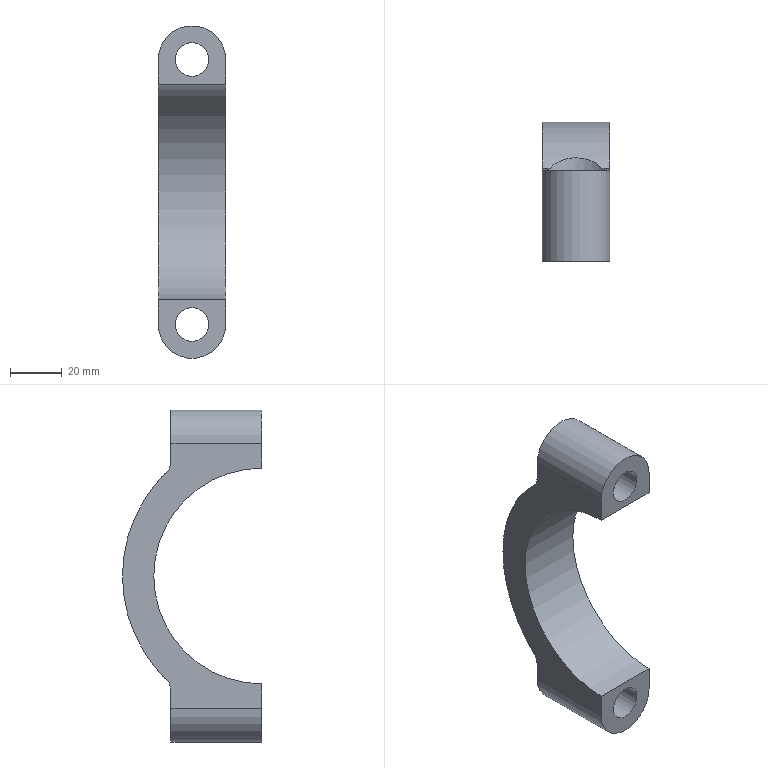Part | NX | features BREP 1 | 1 solid | 22 faces | box 26 x 53.534 x 128 mm | volume 59210 mm3 | cylinder 14 | plane 6 | cone 2 | commonest cylinder face diameters 12.88 x4 24.875 x2 26 x2 27.248 x2 28 x2 82.96 x1
STEP:
#1=CARTESIAN_POINT('',(119.64,34.36,51.));
#2=VERTEX_POINT('',#1);
#3=CARTESIAN_POINT('',(106.76,34.36,51.));
#4=VERTEX_POINT('',#3);
#5=CARTESIAN_POINT('',(113.2,34.36,51.));
#6=DIRECTION('',(0.,1.,0.));
#7=DIRECTION('',(-1.,0.,0.));
#8=AXIS2_PLACEMENT_3D('',#5,#6,#7);
#9=CIRCLE('',#8,6.44);
#10=EDGE_CURVE('',#2,#4,#9,.T.);
#11=ORIENTED_EDGE('',*,*,#10,.F.);
#12=CARTESIAN_POINT('',(120.14,34.86,51.));
#13=VERTEX_POINT('',#12);
#14=CARTESIAN_POINT('',(119.64,34.36,51.));
#15=DIRECTION('',(0.7071,0.7071,0.));
#16=VECTOR('',#15,1000.);
#17=LINE('',#14,#16);
#18=EDGE_CURVE('',#13,#2,#17,.F.);
#19=ORIENTED_EDGE('',*,*,#18,.F.);
#20=CARTESIAN_POINT('',(106.26,34.86,51.));
#21=VERTEX_POINT('',#20);
#22=CARTESIAN_POINT('',(113.2,34.86,51.));
#23=DIRECTION('',(0.,-1.,0.));
#24=DIRECTION('',(-1.,0.,0.));
#25=AXIS2_PLACEMENT_3D('',#22,#23,#24);
#26=CIRCLE('',#25,6.94);
#27=EDGE_CURVE('',#21,#13,#26,.T.);
#28=ORIENTED_EDGE('',*,*,#27,.F.);
#29=CARTESIAN_POINT('',(106.76,34.36,51.));
#30=DIRECTION('',(-0.7071,0.7071,0.));
#31=VECTOR('',#30,1000.);
#32=LINE('',#29,#31);
#33=EDGE_CURVE('',#21,#4,#32,.F.);
#34=ORIENTED_EDGE('',*,*,#33,.T.);
#35=EDGE_LOOP('',(#11,#19,#28,#34));
#36=FACE_BOUND('',#35,.T.);
#37=CARTESIAN_POINT('',(113.2,34.36,51.));
#38=DIRECTION('',(0.,1.,0.));
#39=DIRECTION('',(1.,0.,0.));
#40=AXIS2_PLACEMENT_3D('',#37,#38,#39);
#41=CONICAL_SURFACE('',#40,6.44,0.7854);
#42=ADVANCED_FACE('',(#36),#41,.F.);
#43=ORIENTED_EDGE('',*,*,#10,.T.);
#44=CARTESIAN_POINT('',(106.76,0.,51.));
#45=VERTEX_POINT('',#44);
#46=CARTESIAN_POINT('',(106.76,0.,51.));
#47=DIRECTION('',(0.,-1.,0.));
#48=VECTOR('',#47,1000.);
#49=LINE('',#46,#48);
#50=EDGE_CURVE('',#4,#45,#49,.T.);
#51=ORIENTED_EDGE('',*,*,#50,.T.);
#52=CARTESIAN_POINT('',(119.64,0.,51.));
#53=VERTEX_POINT('',#52);
#54=CARTESIAN_POINT('',(113.2,0.,51.));
#55=DIRECTION('',(0.,-1.,0.));
#56=DIRECTION('',(1.,0.,0.));
#57=AXIS2_PLACEMENT_3D('',#54,#55,#56);
#58=CIRCLE('',#57,6.44);
#59=EDGE_CURVE('',#45,#53,#58,.T.);
#60=ORIENTED_EDGE('',*,*,#59,.T.);
#61=CARTESIAN_POINT('',(119.64,0.,51.));
#62=DIRECTION('',(0.,-1.,0.));
#63=VECTOR('',#62,1000.);
#64=LINE('',#61,#63);
#65=EDGE_CURVE('',#2,#53,#64,.T.);
#66=ORIENTED_EDGE('',*,*,#65,.F.);
#67=EDGE_LOOP('',(#43,#51,#60,#66));
#68=FACE_BOUND('',#67,.T.);
#69=CARTESIAN_POINT('',(113.2,0.,51.));
#70=DIRECTION('',(0.,-1.,0.));
#71=DIRECTION('',(-1.,0.,0.));
#72=AXIS2_PLACEMENT_3D('',#69,#70,#71);
#73=CYLINDRICAL_SURFACE('',#72,6.44);
#74=ADVANCED_FACE('',(#68),#73,.F.);
#75=CARTESIAN_POINT('',(119.64,34.86,-51.));
#76=VERTEX_POINT('',#75);
#77=CARTESIAN_POINT('',(106.76,34.86,-51.));
#78=VERTEX_POINT('',#77);
#79=CARTESIAN_POINT('',(113.2,34.86,-51.));
#80=DIRECTION('',(0.,1.,0.));
#81=DIRECTION('',(-1.,0.,0.));
#82=AXIS2_PLACEMENT_3D('',#79,#80,#81);
#83=CIRCLE('',#82,6.44);
#84=EDGE_CURVE('',#76,#78,#83,.T.);
#85=ORIENTED_EDGE('',*,*,#84,.T.);
#86=CARTESIAN_POINT('',(106.76,0.,-51.));
#87=VERTEX_POINT('',#86);
#88=CARTESIAN_POINT('',(106.76,0.,-51.));
#89=DIRECTION('',(0.,-1.,0.));
#90=VECTOR('',#89,1000.);
#91=LINE('',#88,#90);
#92=EDGE_CURVE('',#78,#87,#91,.T.);
#93=ORIENTED_EDGE('',*,*,#92,.T.);
#94=CARTESIAN_POINT('',(119.64,0.,-51.));
#95=VERTEX_POINT('',#94);
#96=CARTESIAN_POINT('',(113.2,0.,-51.));
#97=DIRECTION('',(0.,-1.,0.));
#98=DIRECTION('',(1.,0.,0.));
#99=AXIS2_PLACEMENT_3D('',#96,#97,#98);
#100=CIRCLE('',#99,6.44);
#101=EDGE_CURVE('',#87,#95,#100,.T.);
#102=ORIENTED_EDGE('',*,*,#101,.T.);
#103=CARTESIAN_POINT('',(119.64,0.,-51.));
#104=DIRECTION('',(0.,-1.,0.));
#105=VECTOR('',#104,1000.);
#106=LINE('',#103,#105);
#107=EDGE_CURVE('',#76,#95,#106,.T.);
#108=ORIENTED_EDGE('',*,*,#107,.F.);
#109=EDGE_LOOP('',(#85,#93,#102,#108));
#110=FACE_BOUND('',#109,.T.);
#111=CARTESIAN_POINT('',(113.2,0.,-51.));
#112=DIRECTION('',(0.,-1.,0.));
#113=DIRECTION('',(-1.,0.,0.));
#114=AXIS2_PLACEMENT_3D('',#111,#112,#113);
#115=CYLINDRICAL_SURFACE('',#114,6.44);
#116=ADVANCED_FACE('',(#110),#115,.F.);
#117=CARTESIAN_POINT('',(113.2,0.,51.));
#118=DIRECTION('',(0.,-1.,0.));
#119=DIRECTION('',(1.,0.,0.));
#120=AXIS2_PLACEMENT_3D('',#117,#118,#119);
#121=CIRCLE('',#120,6.44);
#122=EDGE_CURVE('',#53,#45,#121,.T.);
#123=ORIENTED_EDGE('',*,*,#122,.F.);
#124=ORIENTED_EDGE('',*,*,#59,.F.);
#125=EDGE_LOOP('',(#123,#124));
#126=FACE_BOUND('',#125,.T.);
#127=CARTESIAN_POINT('',(100.2,0.,51.));
#128=VERTEX_POINT('',#127);
#129=CARTESIAN_POINT('',(100.2,0.,41.48));
#130=VERTEX_POINT('',#129);
#131=CARTESIAN_POINT('',(100.2,0.,0.));
#132=DIRECTION('',(0.,0.,-1.));
#133=VECTOR('',#132,1000.);
#134=LINE('',#131,#133);
#135=EDGE_CURVE('',#128,#130,#134,.T.);
#136=ORIENTED_EDGE('',*,*,#135,.T.);
#137=CARTESIAN_POINT('',(126.2,0.,41.48));
#138=VERTEX_POINT('',#137);
#139=CARTESIAN_POINT('',(126.2,0.,41.48));
#140=DIRECTION('',(1.,0.,0.));
#141=VECTOR('',#140,1000.);
#142=LINE('',#139,#141);
#143=EDGE_CURVE('',#130,#138,#142,.T.);
#144=ORIENTED_EDGE('',*,*,#143,.T.);
#145=CARTESIAN_POINT('',(126.2,0.,51.));
#146=VERTEX_POINT('',#145);
#147=CARTESIAN_POINT('',(126.2,0.,0.));
#148=DIRECTION('',(0.,0.,1.));
#149=VECTOR('',#148,1000.);
#150=LINE('',#147,#149);
#151=EDGE_CURVE('',#138,#146,#150,.T.);
#152=ORIENTED_EDGE('',*,*,#151,.T.);
#153=CARTESIAN_POINT('',(113.2,0.,51.));
#154=DIRECTION('',(0.,-1.,0.));
#155=DIRECTION('',(-1.,0.,0.));
#156=AXIS2_PLACEMENT_3D('',#153,#154,#155);
#157=CIRCLE('',#156,13.);
#158=EDGE_CURVE('',#146,#128,#157,.T.);
#159=ORIENTED_EDGE('',*,*,#158,.T.);
#160=EDGE_LOOP('',(#136,#144,#152,#159));
#161=FACE_BOUND('',#160,.T.);
#162=CARTESIAN_POINT('',(113.2,0.,51.));
#163=DIRECTION('',(0.,1.,0.));
#164=DIRECTION('',(1.,0.,0.));
#165=AXIS2_PLACEMENT_3D('',#162,#163,#164);
#166=PLANE('',#165);
#167=ADVANCED_FACE('',(#126,#161),#166,.F.);
#168=CARTESIAN_POINT('',(126.2,0.,-41.48));
#169=VERTEX_POINT('',#168);
#170=CARTESIAN_POINT('',(126.2,0.,0.));
#171=DIRECTION('',(1.,0.,0.));
#172=DIRECTION('',(0.,0.,-1.));
#173=AXIS2_PLACEMENT_3D('',#170,#171,#172);
#174=CIRCLE('',#173,41.48);
#175=EDGE_CURVE('',#169,#138,#174,.T.);
#176=ORIENTED_EDGE('',*,*,#175,.F.);
#177=CARTESIAN_POINT('',(126.2,0.,-51.));
#178=VERTEX_POINT('',#177);
#179=CARTESIAN_POINT('',(126.2,0.,0.));
#180=DIRECTION('',(0.,0.,1.));
#181=VECTOR('',#180,1000.);
#182=LINE('',#179,#181);
#183=EDGE_CURVE('',#178,#169,#182,.T.);
#184=ORIENTED_EDGE('',*,*,#183,.F.);
#185=CARTESIAN_POINT('',(126.2,34.86,-51.));
#186=VERTEX_POINT('',#185);
#187=CARTESIAN_POINT('',(126.2,0.,-51.));
#188=DIRECTION('',(0.,1.,0.));
#189=VECTOR('',#188,1000.);
#190=LINE('',#187,#189);
#191=EDGE_CURVE('',#178,#186,#190,.T.);
#192=ORIENTED_EDGE('',*,*,#191,.T.);
#193=CARTESIAN_POINT('',(126.2,34.86,-45.263));
#194=VERTEX_POINT('',#193);
#195=CARTESIAN_POINT('',(126.2,34.86,0.));
#196=DIRECTION('',(0.,0.,1.));
#197=VECTOR('',#196,1000.);
#198=LINE('',#195,#197);
#199=EDGE_CURVE('',#186,#194,#198,.T.);
#200=ORIENTED_EDGE('',*,*,#199,.T.);
#201=CARTESIAN_POINT('',(126.2,35.762,-40.679));
#202=VERTEX_POINT('',#201);
#203=CARTESIAN_POINT('',(126.2,48.481,-45.563));
#204=DIRECTION('',(-1.,0.,0.));
#205=DIRECTION('',(0.,0.,1.));
#206=AXIS2_PLACEMENT_3D('',#203,#204,#205);
#207=CIRCLE('',#206,13.624);
#208=EDGE_CURVE('',#194,#202,#207,.T.);
#209=ORIENTED_EDGE('',*,*,#208,.T.);
#210=CARTESIAN_POINT('',(126.2,35.762,40.679));
#211=VERTEX_POINT('',#210);
#212=CARTESIAN_POINT('',(126.2,-1.908,-0.0001081));
#213=DIRECTION('',(1.,0.,0.));
#214=DIRECTION('',(0.,0.,-1.));
#215=AXIS2_PLACEMENT_3D('',#212,#213,#214);
#216=CIRCLE('',#215,55.442);
#217=EDGE_CURVE('',#202,#211,#216,.T.);
#218=ORIENTED_EDGE('',*,*,#217,.T.);
#219=CARTESIAN_POINT('',(126.2,34.86,45.329));
#220=VERTEX_POINT('',#219);
#221=CARTESIAN_POINT('',(126.2,47.298,45.329));
#222=DIRECTION('',(1.,0.,0.));
#223=DIRECTION('',(0.,0.,-1.));
#224=AXIS2_PLACEMENT_3D('',#221,#222,#223);
#225=CIRCLE('',#224,12.438);
#226=EDGE_CURVE('',#220,#211,#225,.T.);
#227=ORIENTED_EDGE('',*,*,#226,.F.);
#228=CARTESIAN_POINT('',(126.2,34.86,51.));
#229=VERTEX_POINT('',#228);
#230=CARTESIAN_POINT('',(126.2,34.86,0.));
#231=DIRECTION('',(0.,0.,1.));
#232=VECTOR('',#231,1000.);
#233=LINE('',#230,#232);
#234=EDGE_CURVE('',#220,#229,#233,.T.);
#235=ORIENTED_EDGE('',*,*,#234,.T.);
#236=CARTESIAN_POINT('',(126.2,0.,51.));
#237=DIRECTION('',(0.,1.,0.));
#238=VECTOR('',#237,1000.);
#239=LINE('',#236,#238);
#240=EDGE_CURVE('',#146,#229,#239,.T.);
#241=ORIENTED_EDGE('',*,*,#240,.F.);
#242=ORIENTED_EDGE('',*,*,#151,.F.);
#243=EDGE_LOOP('',(#176,#184,#192,#200,#209,#218,#227,#235,#241,#242));
#244=FACE_BOUND('',#243,.T.);
#245=CARTESIAN_POINT('',(126.2,48.481,-45.563));
#246=DIRECTION('',(-1.,0.,0.));
#247=DIRECTION('',(0.,0.,-1.));
#248=AXIS2_PLACEMENT_3D('',#245,#246,#247);
#249=PLANE('',#248);
#250=ADVANCED_FACE('',(#244),#249,.F.);
#251=CARTESIAN_POINT('',(100.2,0.,-41.48));
#252=VERTEX_POINT('',#251);
#253=CARTESIAN_POINT('',(100.2,0.,-51.));
#254=VERTEX_POINT('',#253);
#255=CARTESIAN_POINT('',(100.2,0.,0.));
#256=DIRECTION('',(0.,0.,-1.));
#257=VECTOR('',#256,1000.);
#258=LINE('',#255,#257);
#259=EDGE_CURVE('',#252,#254,#258,.T.);
#260=ORIENTED_EDGE('',*,*,#259,.F.);
#261=CARTESIAN_POINT('',(100.2,0.,0.));
#262=DIRECTION('',(1.,0.,0.));
#263=DIRECTION('',(0.,0.,-1.));
#264=AXIS2_PLACEMENT_3D('',#261,#262,#263);
#265=CIRCLE('',#264,41.48);
#266=EDGE_CURVE('',#252,#130,#265,.T.);
#267=ORIENTED_EDGE('',*,*,#266,.T.);
#268=ORIENTED_EDGE('',*,*,#135,.F.);
#269=CARTESIAN_POINT('',(100.2,34.86,51.));
#270=VERTEX_POINT('',#269);
#271=CARTESIAN_POINT('',(100.2,0.,51.));
#272=DIRECTION('',(0.,1.,0.));
#273=VECTOR('',#272,1000.);
#274=LINE('',#271,#273);
#275=EDGE_CURVE('',#128,#270,#274,.T.);
#276=ORIENTED_EDGE('',*,*,#275,.T.);
#277=CARTESIAN_POINT('',(100.2,34.86,45.329));
#278=VERTEX_POINT('',#277);
#279=CARTESIAN_POINT('',(100.2,34.86,0.));
#280=DIRECTION('',(0.,0.,-1.));
#281=VECTOR('',#280,1000.);
#282=LINE('',#279,#281);
#283=EDGE_CURVE('',#270,#278,#282,.T.);
#284=ORIENTED_EDGE('',*,*,#283,.T.);
#285=CARTESIAN_POINT('',(100.2,35.762,40.679));
#286=VERTEX_POINT('',#285);
#287=CARTESIAN_POINT('',(100.2,47.298,45.329));
#288=DIRECTION('',(1.,0.,0.));
#289=DIRECTION('',(0.,0.,-1.));
#290=AXIS2_PLACEMENT_3D('',#287,#288,#289);
#291=CIRCLE('',#290,12.438);
#292=EDGE_CURVE('',#278,#286,#291,.T.);
#293=ORIENTED_EDGE('',*,*,#292,.T.);
#294=CARTESIAN_POINT('',(100.2,35.762,-40.679));
#295=VERTEX_POINT('',#294);
#296=CARTESIAN_POINT('',(100.2,-1.908,-0.0001081));
#297=DIRECTION('',(1.,0.,0.));
#298=DIRECTION('',(0.,0.,-1.));
#299=AXIS2_PLACEMENT_3D('',#296,#297,#298);
#300=CIRCLE('',#299,55.442);
#301=EDGE_CURVE('',#295,#286,#300,.T.);
#302=ORIENTED_EDGE('',*,*,#301,.F.);
#303=CARTESIAN_POINT('',(100.2,34.86,-45.263));
#304=VERTEX_POINT('',#303);
#305=CARTESIAN_POINT('',(100.2,48.481,-45.563));
#306=DIRECTION('',(-1.,0.,0.));
#307=DIRECTION('',(0.,0.,1.));
#308=AXIS2_PLACEMENT_3D('',#305,#306,#307);
#309=CIRCLE('',#308,13.624);
#310=EDGE_CURVE('',#304,#295,#309,.T.);
#311=ORIENTED_EDGE('',*,*,#310,.F.);
#312=CARTESIAN_POINT('',(100.2,34.86,-51.));
#313=VERTEX_POINT('',#312);
#314=CARTESIAN_POINT('',(100.2,34.86,0.));
#315=DIRECTION('',(0.,0.,-1.));
#316=VECTOR('',#315,1000.);
#317=LINE('',#314,#316);
#318=EDGE_CURVE('',#304,#313,#317,.T.);
#319=ORIENTED_EDGE('',*,*,#318,.T.);
#320=CARTESIAN_POINT('',(100.2,0.,-51.));
#321=DIRECTION('',(0.,1.,0.));
#322=VECTOR('',#321,1000.);
#323=LINE('',#320,#322);
#324=EDGE_CURVE('',#254,#313,#323,.T.);
#325=ORIENTED_EDGE('',*,*,#324,.F.);
#326=EDGE_LOOP('',(#260,#267,#268,#276,#284,#293,#302,#311,#319,#325));
#327=FACE_BOUND('',#326,.T.);
#328=CARTESIAN_POINT('',(100.2,48.481,-45.563));
#329=DIRECTION('',(-1.,0.,0.));
#330=DIRECTION('',(0.,0.,-1.));
#331=AXIS2_PLACEMENT_3D('',#328,#329,#330);
#332=PLANE('',#331);
#333=ADVANCED_FACE('',(#327),#332,.T.);
#334=ORIENTED_EDGE('',*,*,#292,.F.);
#335=CARTESIAN_POINT('',(103.247,35.762,40.679));
#336=VERTEX_POINT('',#335);
#337=CARTESIAN_POINT('',(100.2,34.86,45.329));
#338=CARTESIAN_POINT('',(100.91,34.86,43.552));
#339=CARTESIAN_POINT('',(101.957,35.236,41.984));
#340=CARTESIAN_POINT('',(103.247,35.762,40.679));
#341=B_SPLINE_CURVE_WITH_KNOTS('',3,(#337,#338,#339,#340),.UNSPECIFIED.,.F.,.F.,(4,4),(0.,0.005644),.UNSPECIFIED.);
#342=EDGE_CURVE('',#278,#336,#341,.T.);
#343=ORIENTED_EDGE('',*,*,#342,.T.);
#344=CARTESIAN_POINT('',(100.2,35.762,40.679));
#345=DIRECTION('',(1.,0.,0.));
#346=VECTOR('',#345,1000.);
#347=LINE('',#344,#346);
#348=EDGE_CURVE('',#286,#336,#347,.T.);
#349=ORIENTED_EDGE('',*,*,#348,.F.);
#350=EDGE_LOOP('',(#334,#343,#349));
#351=FACE_BOUND('',#350,.T.);
#352=CARTESIAN_POINT('',(100.2,47.298,45.329));
#353=DIRECTION('',(1.,0.,0.));
#354=DIRECTION('',(0.,0.,1.));
#355=AXIS2_PLACEMENT_3D('',#352,#353,#354);
#356=CYLINDRICAL_SURFACE('',#355,12.438);
#357=ADVANCED_FACE('',(#351),#356,.F.);
#358=CARTESIAN_POINT('',(103.182,35.762,-40.679));
#359=VERTEX_POINT('',#358);
#360=CARTESIAN_POINT('',(100.2,34.86,-45.263));
#361=CARTESIAN_POINT('',(100.898,34.898,-43.517));
#362=CARTESIAN_POINT('',(101.918,35.265,-41.975));
#363=CARTESIAN_POINT('',(103.182,35.762,-40.679));
#364=B_SPLINE_CURVE_WITH_KNOTS('',3,(#360,#361,#362,#363),.UNSPECIFIED.,.F.,.F.,(4,4),(0.,0.005551),.UNSPECIFIED.);
#365=EDGE_CURVE('',#304,#359,#364,.T.);
#366=ORIENTED_EDGE('',*,*,#365,.F.);
#367=ORIENTED_EDGE('',*,*,#310,.T.);
#368=CARTESIAN_POINT('',(100.2,35.762,-40.679));
#369=DIRECTION('',(1.,0.,0.));
#370=VECTOR('',#369,1000.);
#371=LINE('',#368,#370);
#372=EDGE_CURVE('',#295,#359,#371,.T.);
#373=ORIENTED_EDGE('',*,*,#372,.T.);
#374=EDGE_LOOP('',(#366,#367,#373));
#375=FACE_BOUND('',#374,.T.);
#376=CARTESIAN_POINT('',(100.2,48.481,-45.563));
#377=DIRECTION('',(1.,0.,0.));
#378=DIRECTION('',(0.,0.,1.));
#379=AXIS2_PLACEMENT_3D('',#376,#377,#378);
#380=CYLINDRICAL_SURFACE('',#379,13.624);
#381=ADVANCED_FACE('',(#375),#380,.F.);
#382=ORIENTED_EDGE('',*,*,#175,.T.);
#383=ORIENTED_EDGE('',*,*,#143,.F.);
#384=ORIENTED_EDGE('',*,*,#266,.F.);
#385=CARTESIAN_POINT('',(126.2,0.,-41.48));
#386=DIRECTION('',(-1.,0.,0.));
#387=VECTOR('',#386,1000.);
#388=LINE('',#385,#387);
#389=EDGE_CURVE('',#169,#252,#388,.T.);
#390=ORIENTED_EDGE('',*,*,#389,.F.);
#391=EDGE_LOOP('',(#382,#383,#384,#390));
#392=FACE_BOUND('',#391,.T.);
#393=CARTESIAN_POINT('',(100.2,0.,0.));
#394=DIRECTION('',(1.,0.,0.));
#395=DIRECTION('',(0.,0.,1.));
#396=AXIS2_PLACEMENT_3D('',#393,#394,#395);
#397=CYLINDRICAL_SURFACE('',#396,41.48);
#398=ADVANCED_FACE('',(#392),#397,.F.);
#399=CARTESIAN_POINT('',(123.153,35.762,40.679));
#400=VERTEX_POINT('',#399);
#401=CARTESIAN_POINT('',(100.2,35.762,40.679));
#402=DIRECTION('',(1.,0.,0.));
#403=VECTOR('',#402,1000.);
#404=LINE('',#401,#403);
#405=EDGE_CURVE('',#400,#211,#404,.T.);
#406=ORIENTED_EDGE('',*,*,#405,.F.);
#407=CARTESIAN_POINT('',(123.153,35.762,40.679));
#408=CARTESIAN_POINT('',(124.441,35.237,41.982));
#409=CARTESIAN_POINT('',(125.491,34.86,43.555));
#410=CARTESIAN_POINT('',(126.2,34.86,45.329));
#411=B_SPLINE_CURVE_WITH_KNOTS('',3,(#407,#408,#409,#410),.UNSPECIFIED.,.F.,.F.,(4,4),(0.,0.00565),.UNSPECIFIED.);
#412=EDGE_CURVE('',#400,#220,#411,.T.);
#413=ORIENTED_EDGE('',*,*,#412,.T.);
#414=ORIENTED_EDGE('',*,*,#226,.T.);
#415=EDGE_LOOP('',(#406,#413,#414));
#416=FACE_BOUND('',#415,.T.);
#417=CARTESIAN_POINT('',(100.2,47.298,45.329));
#418=DIRECTION('',(1.,0.,0.));
#419=DIRECTION('',(0.,0.,1.));
#420=AXIS2_PLACEMENT_3D('',#417,#418,#419);
#421=CYLINDRICAL_SURFACE('',#420,12.438);
#422=ADVANCED_FACE('',(#416),#421,.F.);
#423=CARTESIAN_POINT('',(123.218,35.762,-40.679));
#424=VERTEX_POINT('',#423);
#425=CARTESIAN_POINT('',(103.182,35.762,-40.679));
#426=CARTESIAN_POINT('',(104.306,37.004,-39.529));
#427=CARTESIAN_POINT('',(107.166,39.066,-37.394));
#428=CARTESIAN_POINT('',(113.162,40.254,-35.995));
#429=CARTESIAN_POINT('',(119.23,39.076,-37.383));
#430=CARTESIAN_POINT('',(122.093,37.006,-39.527));
#431=CARTESIAN_POINT('',(123.218,35.762,-40.679));
#432=B_SPLINE_CURVE_WITH_KNOTS('',3,(#425,#426,#427,#428,#429,#430,#431),.UNSPECIFIED.,.F.,.F.,(4,1,1,1,4),(0.,0.006027,0.01205,0.01808,0.02411),.UNSPECIFIED.);
#433=EDGE_CURVE('',#359,#424,#432,.T.);
#434=ORIENTED_EDGE('',*,*,#433,.F.);
#435=ORIENTED_EDGE('',*,*,#372,.F.);
#436=ORIENTED_EDGE('',*,*,#301,.T.);
#437=ORIENTED_EDGE('',*,*,#348,.T.);
#438=CARTESIAN_POINT('',(123.153,35.762,40.679));
#439=CARTESIAN_POINT('',(122.03,36.988,39.544));
#440=CARTESIAN_POINT('',(119.179,39.02,37.442));
#441=CARTESIAN_POINT('',(113.238,40.19,36.07));
#442=CARTESIAN_POINT('',(107.225,39.031,37.431));
#443=CARTESIAN_POINT('',(104.372,36.99,39.542));
#444=CARTESIAN_POINT('',(103.247,35.762,40.679));
#445=B_SPLINE_CURVE_WITH_KNOTS('',3,(#438,#439,#440,#441,#442,#443,#444),.UNSPECIFIED.,.F.,.F.,(4,1,1,1,4),(0.,0.005971,0.01194,0.01791,0.02389),.UNSPECIFIED.);
#446=EDGE_CURVE('',#400,#336,#445,.T.);
#447=ORIENTED_EDGE('',*,*,#446,.F.);
#448=ORIENTED_EDGE('',*,*,#405,.T.);
#449=ORIENTED_EDGE('',*,*,#217,.F.);
#450=CARTESIAN_POINT('',(100.2,35.762,-40.679));
#451=DIRECTION('',(1.,0.,0.));
#452=VECTOR('',#451,1000.);
#453=LINE('',#450,#452);
#454=EDGE_CURVE('',#424,#202,#453,.T.);
#455=ORIENTED_EDGE('',*,*,#454,.F.);
#456=EDGE_LOOP('',(#434,#435,#436,#437,#447,#448,#449,#455));
#457=FACE_BOUND('',#456,.T.);
#458=CARTESIAN_POINT('',(100.2,-1.908,-0.0001081));
#459=DIRECTION('',(1.,0.,0.));
#460=DIRECTION('',(0.,0.,1.));
#461=AXIS2_PLACEMENT_3D('',#458,#459,#460);
#462=CYLINDRICAL_SURFACE('',#461,55.442);
#463=ADVANCED_FACE('',(#457),#462,.T.);
#464=CARTESIAN_POINT('',(123.218,35.762,-40.679));
#465=CARTESIAN_POINT('',(124.48,35.265,-41.973));
#466=CARTESIAN_POINT('',(125.503,34.898,-43.519));
#467=CARTESIAN_POINT('',(126.2,34.86,-45.263));
#468=B_SPLINE_CURVE_WITH_KNOTS('',3,(#464,#465,#466,#467),.UNSPECIFIED.,.F.,.F.,(4,4),(0.,0.005555),.UNSPECIFIED.);
#469=EDGE_CURVE('',#424,#194,#468,.T.);
#470=ORIENTED_EDGE('',*,*,#469,.F.);
#471=ORIENTED_EDGE('',*,*,#454,.T.);
#472=ORIENTED_EDGE('',*,*,#208,.F.);
#473=EDGE_LOOP('',(#470,#471,#472));
#474=FACE_BOUND('',#473,.T.);
#475=CARTESIAN_POINT('',(100.2,48.481,-45.563));
#476=DIRECTION('',(1.,0.,0.));
#477=DIRECTION('',(0.,0.,1.));
#478=AXIS2_PLACEMENT_3D('',#475,#476,#477);
#479=CYLINDRICAL_SURFACE('',#478,13.624);
#480=ADVANCED_FACE('',(#474),#479,.F.);
#481=ORIENTED_EDGE('',*,*,#365,.T.);
#482=ORIENTED_EDGE('',*,*,#433,.T.);
#483=ORIENTED_EDGE('',*,*,#469,.T.);
#484=CARTESIAN_POINT('',(113.2,34.86,-50.459));
#485=DIRECTION('',(0.,-1.,0.));
#486=DIRECTION('',(1.,0.,0.));
#487=AXIS2_PLACEMENT_3D('',#484,#485,#486);
#488=CIRCLE('',#487,14.);
#489=EDGE_CURVE('',#194,#304,#488,.T.);
#490=ORIENTED_EDGE('',*,*,#489,.T.);
#491=EDGE_LOOP('',(#481,#482,#483,#490));
#492=FACE_BOUND('',#491,.T.);
#493=CARTESIAN_POINT('',(113.2,44.86,-50.459));
#494=DIRECTION('',(0.,-1.,0.));
#495=DIRECTION('',(-1.,0.,0.));
#496=AXIS2_PLACEMENT_3D('',#493,#494,#495);
#497=CYLINDRICAL_SURFACE('',#496,14.);
#498=ADVANCED_FACE('',(#492),#497,.F.);
#499=CARTESIAN_POINT('',(113.2,34.86,50.525));
#500=DIRECTION('',(0.,-1.,0.));
#501=DIRECTION('',(1.,0.,0.));
#502=AXIS2_PLACEMENT_3D('',#499,#500,#501);
#503=CIRCLE('',#502,14.);
#504=EDGE_CURVE('',#278,#220,#503,.T.);
#505=ORIENTED_EDGE('',*,*,#504,.T.);
#506=ORIENTED_EDGE('',*,*,#412,.F.);
#507=ORIENTED_EDGE('',*,*,#446,.T.);
#508=ORIENTED_EDGE('',*,*,#342,.F.);
#509=EDGE_LOOP('',(#505,#506,#507,#508));
#510=FACE_BOUND('',#509,.T.);
#511=CARTESIAN_POINT('',(113.2,44.86,50.525));
#512=DIRECTION('',(0.,-1.,0.));
#513=DIRECTION('',(-1.,0.,0.));
#514=AXIS2_PLACEMENT_3D('',#511,#512,#513);
#515=CYLINDRICAL_SURFACE('',#514,14.);
#516=ADVANCED_FACE('',(#510),#515,.F.);
#517=ORIENTED_EDGE('',*,*,#84,.F.);
#518=CARTESIAN_POINT('',(113.2,34.86,-51.));
#519=DIRECTION('',(0.,1.,0.));
#520=DIRECTION('',(-1.,0.,0.));
#521=AXIS2_PLACEMENT_3D('',#518,#519,#520);
#522=CIRCLE('',#521,6.44);
#523=EDGE_CURVE('',#78,#76,#522,.T.);
#524=ORIENTED_EDGE('',*,*,#523,.F.);
#525=EDGE_LOOP('',(#517,#524));
#526=FACE_BOUND('',#525,.T.);
#527=ORIENTED_EDGE('',*,*,#489,.F.);
#528=ORIENTED_EDGE('',*,*,#199,.F.);
#529=CARTESIAN_POINT('',(113.2,34.86,-51.));
#530=DIRECTION('',(0.,-1.,0.));
#531=DIRECTION('',(1.,0.,0.));
#532=AXIS2_PLACEMENT_3D('',#529,#530,#531);
#533=CIRCLE('',#532,13.);
#534=EDGE_CURVE('',#313,#186,#533,.T.);
#535=ORIENTED_EDGE('',*,*,#534,.F.);
#536=ORIENTED_EDGE('',*,*,#318,.F.);
#537=EDGE_LOOP('',(#527,#528,#535,#536));
#538=FACE_BOUND('',#537,.T.);
#539=CARTESIAN_POINT('',(113.2,34.86,51.));
#540=DIRECTION('',(0.,1.,0.));
#541=DIRECTION('',(1.,0.,0.));
#542=AXIS2_PLACEMENT_3D('',#539,#540,#541);
#543=PLANE('',#542);
#544=ADVANCED_FACE('',(#526,#538),#543,.T.);
#545=ORIENTED_EDGE('',*,*,#27,.T.);
#546=CARTESIAN_POINT('',(113.2,34.86,51.));
#547=DIRECTION('',(0.,-1.,0.));
#548=DIRECTION('',(-1.,0.,0.));
#549=AXIS2_PLACEMENT_3D('',#546,#547,#548);
#550=CIRCLE('',#549,6.94);
#551=EDGE_CURVE('',#13,#21,#550,.T.);
#552=ORIENTED_EDGE('',*,*,#551,.T.);
#553=EDGE_LOOP('',(#545,#552));
#554=FACE_BOUND('',#553,.T.);
#555=ORIENTED_EDGE('',*,*,#504,.F.);
#556=ORIENTED_EDGE('',*,*,#283,.F.);
#557=CARTESIAN_POINT('',(113.2,34.86,51.));
#558=DIRECTION('',(0.,-1.,0.));
#559=DIRECTION('',(-1.,0.,0.));
#560=AXIS2_PLACEMENT_3D('',#557,#558,#559);
#561=CIRCLE('',#560,13.);
#562=EDGE_CURVE('',#229,#270,#561,.T.);
#563=ORIENTED_EDGE('',*,*,#562,.F.);
#564=ORIENTED_EDGE('',*,*,#234,.F.);
#565=EDGE_LOOP('',(#555,#556,#563,#564));
#566=FACE_BOUND('',#565,.T.);
#567=CARTESIAN_POINT('',(113.2,34.86,51.));
#568=DIRECTION('',(0.,1.,0.));
#569=DIRECTION('',(1.,0.,0.));
#570=AXIS2_PLACEMENT_3D('',#567,#568,#569);
#571=PLANE('',#570);
#572=ADVANCED_FACE('',(#554,#566),#571,.T.);
#573=ORIENTED_EDGE('',*,*,#534,.T.);
#574=ORIENTED_EDGE('',*,*,#191,.F.);
#575=CARTESIAN_POINT('',(113.2,0.,-51.));
#576=DIRECTION('',(0.,-1.,0.));
#577=DIRECTION('',(1.,0.,0.));
#578=AXIS2_PLACEMENT_3D('',#575,#576,#577);
#579=CIRCLE('',#578,13.);
#580=EDGE_CURVE('',#254,#178,#579,.T.);
#581=ORIENTED_EDGE('',*,*,#580,.F.);
#582=ORIENTED_EDGE('',*,*,#324,.T.);
#583=EDGE_LOOP('',(#573,#574,#581,#582));
#584=FACE_BOUND('',#583,.T.);
#585=CARTESIAN_POINT('',(113.2,0.,-51.));
#586=DIRECTION('',(0.,1.,0.));
#587=DIRECTION('',(1.,0.,0.));
#588=AXIS2_PLACEMENT_3D('',#585,#586,#587);
#589=CYLINDRICAL_SURFACE('',#588,13.);
#590=ADVANCED_FACE('',(#584),#589,.T.);
#591=ORIENTED_EDGE('',*,*,#562,.T.);
#592=ORIENTED_EDGE('',*,*,#275,.F.);
#593=ORIENTED_EDGE('',*,*,#158,.F.);
#594=ORIENTED_EDGE('',*,*,#240,.T.);
#595=EDGE_LOOP('',(#591,#592,#593,#594));
#596=FACE_BOUND('',#595,.T.);
#597=CARTESIAN_POINT('',(113.2,0.,51.));
#598=DIRECTION('',(0.,1.,0.));
#599=DIRECTION('',(1.,0.,0.));
#600=AXIS2_PLACEMENT_3D('',#597,#598,#599);
#601=CYLINDRICAL_SURFACE('',#600,13.);
#602=ADVANCED_FACE('',(#596),#601,.T.);
#603=CARTESIAN_POINT('',(113.2,0.,-51.));
#604=DIRECTION('',(0.,-1.,0.));
#605=DIRECTION('',(1.,0.,0.));
#606=AXIS2_PLACEMENT_3D('',#603,#604,#605);
#607=CIRCLE('',#606,6.44);
#608=EDGE_CURVE('',#95,#87,#607,.T.);
#609=ORIENTED_EDGE('',*,*,#608,.F.);
#610=ORIENTED_EDGE('',*,*,#101,.F.);
#611=EDGE_LOOP('',(#609,#610));
#612=FACE_BOUND('',#611,.T.);
#613=ORIENTED_EDGE('',*,*,#183,.T.);
#614=ORIENTED_EDGE('',*,*,#389,.T.);
#615=ORIENTED_EDGE('',*,*,#259,.T.);
#616=ORIENTED_EDGE('',*,*,#580,.T.);
#617=EDGE_LOOP('',(#613,#614,#615,#616));
#618=FACE_BOUND('',#617,.T.);
#619=CARTESIAN_POINT('',(113.2,0.,51.));
#620=DIRECTION('',(0.,1.,0.));
#621=DIRECTION('',(1.,0.,0.));
#622=AXIS2_PLACEMENT_3D('',#619,#620,#621);
#623=PLANE('',#622);
#624=ADVANCED_FACE('',(#612,#618),#623,.F.);
#625=ORIENTED_EDGE('',*,*,#92,.F.);
#626=ORIENTED_EDGE('',*,*,#523,.T.);
#627=ORIENTED_EDGE('',*,*,#107,.T.);
#628=ORIENTED_EDGE('',*,*,#608,.T.);
#629=EDGE_LOOP('',(#625,#626,#627,#628));
#630=FACE_BOUND('',#629,.T.);
#631=CARTESIAN_POINT('',(113.2,0.,-51.));
#632=DIRECTION('',(0.,-1.,0.));
#633=DIRECTION('',(-1.,0.,0.));
#634=AXIS2_PLACEMENT_3D('',#631,#632,#633);
#635=CYLINDRICAL_SURFACE('',#634,6.44);
#636=ADVANCED_FACE('',(#630),#635,.F.);
#637=ORIENTED_EDGE('',*,*,#50,.F.);
#638=CARTESIAN_POINT('',(113.2,34.36,51.));
#639=DIRECTION('',(0.,1.,0.));
#640=DIRECTION('',(-1.,0.,0.));
#641=AXIS2_PLACEMENT_3D('',#638,#639,#640);
#642=CIRCLE('',#641,6.44);
#643=EDGE_CURVE('',#4,#2,#642,.T.);
#644=ORIENTED_EDGE('',*,*,#643,.T.);
#645=ORIENTED_EDGE('',*,*,#65,.T.);
#646=ORIENTED_EDGE('',*,*,#122,.T.);
#647=EDGE_LOOP('',(#637,#644,#645,#646));
#648=FACE_BOUND('',#647,.T.);
#649=CARTESIAN_POINT('',(113.2,0.,51.));
#650=DIRECTION('',(0.,-1.,0.));
#651=DIRECTION('',(-1.,0.,0.));
#652=AXIS2_PLACEMENT_3D('',#649,#650,#651);
#653=CYLINDRICAL_SURFACE('',#652,6.44);
#654=ADVANCED_FACE('',(#648),#653,.F.);
#655=ORIENTED_EDGE('',*,*,#18,.T.);
#656=ORIENTED_EDGE('',*,*,#643,.F.);
#657=ORIENTED_EDGE('',*,*,#33,.F.);
#658=ORIENTED_EDGE('',*,*,#551,.F.);
#659=EDGE_LOOP('',(#655,#656,#657,#658));
#660=FACE_BOUND('',#659,.T.);
#661=CARTESIAN_POINT('',(113.2,34.36,51.));
#662=DIRECTION('',(0.,1.,0.));
#663=DIRECTION('',(1.,0.,0.));
#664=AXIS2_PLACEMENT_3D('',#661,#662,#663);
#665=CONICAL_SURFACE('',#664,6.44,0.7854);
#666=ADVANCED_FACE('',(#660),#665,.F.);
#667=CLOSED_SHELL('',(#42,#74,#116,#167,#250,#333,#357,#381,#398,#422,#463,#480,#498,#516,#544,#572,#590,#602,#624,#636,#654,#666));
#668=MANIFOLD_SOLID_BREP('',#667);
#669=(LENGTH_UNIT()NAMED_UNIT(*)SI_UNIT(.MILLI.,.METRE.));
#670=UNCERTAINTY_MEASURE_WITH_UNIT(LENGTH_MEASURE(0.0508),#669,'','');
#671=(NAMED_UNIT(*)PLANE_ANGLE_UNIT()SI_UNIT($,.RADIAN.));
#672=(NAMED_UNIT(*)SI_UNIT($,.STERADIAN.)SOLID_ANGLE_UNIT());
#673=(GEOMETRIC_REPRESENTATION_CONTEXT(3)GLOBAL_UNCERTAINTY_ASSIGNED_CONTEXT((#670))GLOBAL_UNIT_ASSIGNED_CONTEXT((#669,#671,#672))REPRESENTATION_CONTEXT('',''));
#674=ADVANCED_BREP_SHAPE_REPRESENTATION('',(#668),#673);